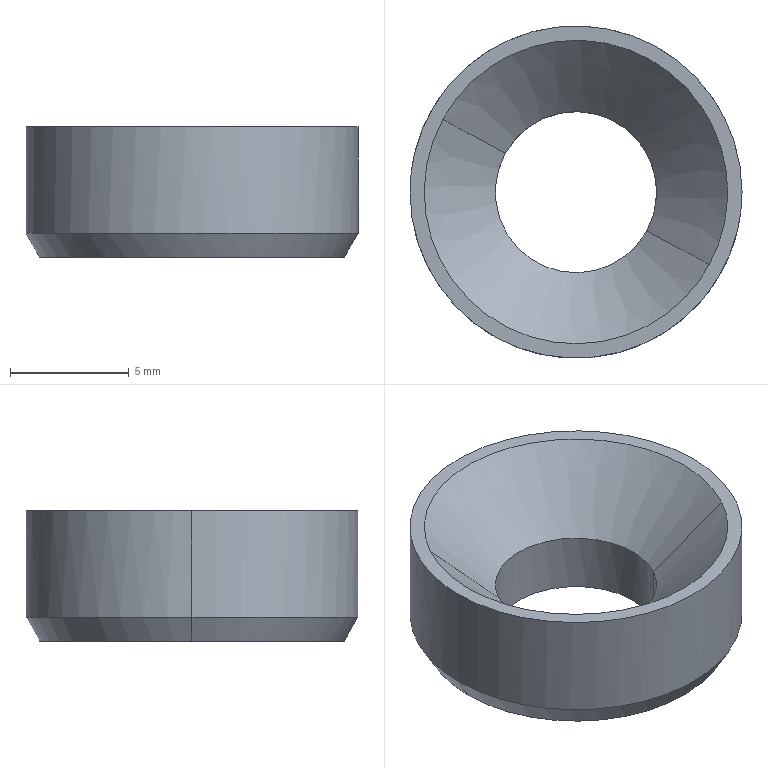Part | CATIA | 1 solid | 10 faces | box 14 x 14 x 5.5 mm | volume 510.162 mm3 | cone 4 | cylinder 4 | plane 2 | commonest cylinder face diameters 6.8 x2 14 x2
STEP:
#1=CARTESIAN_POINT('',(5.617,-3.068,5.5));
#2=VERTEX_POINT('',#1);
#3=CARTESIAN_POINT('',(-5.617,3.068,5.5));
#4=VERTEX_POINT('',#3);
#5=CARTESIAN_POINT('',(0.,0.,5.5));
#6=DIRECTION('',(0.,0.,1.));
#7=AXIS2_PLACEMENT_3D('',#5,#6,$);
#8=CIRCLE('',#7,6.4);
#9=EDGE_CURVE('',#2,#4,#8,.T.);
#10=ORIENTED_EDGE('',*,*,#9,.T.);
#11=CARTESIAN_POINT('',(-2.984,1.63,2.5));
#12=VERTEX_POINT('',#11);
#13=CARTESIAN_POINT('',(-310273.782,169503.34,353554.191));
#14=DIRECTION('',(-0.6205,0.339,0.7071));
#15=VECTOR('',#14,1.);
#16=LINE('',#13,#15);
#17=EDGE_CURVE('',#12,#4,#16,.T.);
#18=ORIENTED_EDGE('',*,*,#17,.F.);
#19=CARTESIAN_POINT('',(2.984,-1.63,2.5));
#20=VERTEX_POINT('',#19);
#21=CARTESIAN_POINT('',(0.,0.,2.5));
#22=DIRECTION('',(0.,0.,1.));
#23=AXIS2_PLACEMENT_3D('',#21,#22,$);
#24=CIRCLE('',#23,3.4);
#25=EDGE_CURVE('',#12,#20,#24,.F.);
#26=ORIENTED_EDGE('',*,*,#25,.T.);
#27=CARTESIAN_POINT('',(310273.782,-169503.34,353554.191));
#28=DIRECTION('',(0.6205,-0.339,0.7071));
#29=VECTOR('',#28,1.);
#30=LINE('',#27,#29);
#31=EDGE_CURVE('',#20,#2,#30,.T.);
#32=ORIENTED_EDGE('',*,*,#31,.T.);
#33=EDGE_LOOP('',(#10,#18,#26,#32));
#34=FACE_OUTER_BOUND('',#33,.T.);
#35=CARTESIAN_POINT('',(0.,0.,2.5));
#36=DIRECTION('',(0.,0.,1.));
#37=DIRECTION('',(0.8776,-0.4794,0.));
#38=AXIS2_PLACEMENT_3D('',#35,#36,#37);
#39=CONICAL_SURFACE('',#38,3.4,0.7854);
#40=ADVANCED_FACE('',(#34),#39,.F.);
#41=CARTESIAN_POINT('',(7.,0.,5.5));
#42=VERTEX_POINT('',#41);
#43=CARTESIAN_POINT('',(-7.,0.,5.5));
#44=VERTEX_POINT('',#43);
#45=CARTESIAN_POINT('',(7.,0.,5.5));
#46=CARTESIAN_POINT('',(7.,0.6481,5.5));
#47=CARTESIAN_POINT('',(6.925,1.296,5.5));
#48=CARTESIAN_POINT('',(6.775,1.933,5.5));
#49=CARTESIAN_POINT('',(6.33,3.159,5.5));
#50=CARTESIAN_POINT('',(5.617,4.252,5.5));
#51=CARTESIAN_POINT('',(5.199,4.755,5.5));
#52=CARTESIAN_POINT('',(4.253,5.654,5.5));
#53=CARTESIAN_POINT('',(3.127,6.313,5.5));
#54=CARTESIAN_POINT('',(2.529,6.576,5.5));
#55=CARTESIAN_POINT('',(1.281,6.958,5.5));
#56=CARTESIAN_POINT('',(-0.02086,7.045,5.5));
#57=CARTESIAN_POINT('',(-0.674,7.013,5.5));
#58=CARTESIAN_POINT('',(-1.961,6.798,5.5));
#59=CARTESIAN_POINT('',(-3.165,6.294,5.5));
#60=CARTESIAN_POINT('',(-3.735,5.974,5.5));
#61=CARTESIAN_POINT('',(-4.79,5.207,5.5));
#62=CARTESIAN_POINT('',(-5.642,4.219,5.5));
#63=CARTESIAN_POINT('',(-6.009,3.677,5.5));
#64=CARTESIAN_POINT('',(-6.547,2.643,5.5));
#65=CARTESIAN_POINT('',(-6.861,1.524,5.5));
#66=CARTESIAN_POINT('',(-6.954,1.02,5.5));
#67=CARTESIAN_POINT('',(-7.,0.5098,5.5));
#68=CARTESIAN_POINT('',(-7.,0.,5.5));
#69=B_SPLINE_CURVE_WITH_KNOTS('',5,(#45,#46,#47,#48,#49,#50,#51,#52,#53,#54,#55,#56,#57,#58,#59,#60,#61,#62,#63,#64,#65,#66,#67,#68),.UNSPECIFIED.,.F.,.U.,(6,3,3,3,3,3,3,6),(0.,4.583,9.165,13.748,18.33,22.913,27.495,31.1),.UNSPECIFIED.);
#70=EDGE_CURVE('',#42,#44,#69,.T.);
#71=ORIENTED_EDGE('',*,*,#70,.T.);
#72=CARTESIAN_POINT('',(-7.,0.,5.5));
#73=CARTESIAN_POINT('',(-7.,-0.6481,5.5));
#74=CARTESIAN_POINT('',(-6.925,-1.296,5.5));
#75=CARTESIAN_POINT('',(-6.775,-1.933,5.5));
#76=CARTESIAN_POINT('',(-6.33,-3.159,5.5));
#77=CARTESIAN_POINT('',(-5.617,-4.252,5.5));
#78=CARTESIAN_POINT('',(-5.199,-4.755,5.5));
#79=CARTESIAN_POINT('',(-4.253,-5.654,5.5));
#80=CARTESIAN_POINT('',(-3.127,-6.313,5.5));
#81=CARTESIAN_POINT('',(-2.529,-6.576,5.5));
#82=CARTESIAN_POINT('',(-1.281,-6.958,5.5));
#83=CARTESIAN_POINT('',(0.02086,-7.045,5.5));
#84=CARTESIAN_POINT('',(0.674,-7.013,5.5));
#85=CARTESIAN_POINT('',(1.961,-6.798,5.5));
#86=CARTESIAN_POINT('',(3.165,-6.294,5.5));
#87=CARTESIAN_POINT('',(3.735,-5.974,5.5));
#88=CARTESIAN_POINT('',(4.79,-5.207,5.5));
#89=CARTESIAN_POINT('',(5.642,-4.219,5.5));
#90=CARTESIAN_POINT('',(6.009,-3.677,5.5));
#91=CARTESIAN_POINT('',(6.547,-2.643,5.5));
#92=CARTESIAN_POINT('',(6.861,-1.524,5.5));
#93=CARTESIAN_POINT('',(6.954,-1.02,5.5));
#94=CARTESIAN_POINT('',(7.,-0.5098,5.5));
#95=CARTESIAN_POINT('',(7.,0.,5.5));
#96=B_SPLINE_CURVE_WITH_KNOTS('',5,(#72,#73,#74,#75,#76,#77,#78,#79,#80,#81,#82,#83,#84,#85,#86,#87,#88,#89,#90,#91,#92,#93,#94,#95),.UNSPECIFIED.,.F.,.U.,(6,3,3,3,3,3,3,6),(0.,4.583,9.165,13.748,18.33,22.913,27.495,31.1),.UNSPECIFIED.);
#97=EDGE_CURVE('',#44,#42,#96,.T.);
#98=ORIENTED_EDGE('',*,*,#97,.T.);
#99=EDGE_LOOP('',(#71,#98));
#100=FACE_OUTER_BOUND('',#99,.T.);
#101=CARTESIAN_POINT('',(-5.617,3.068,5.5));
#102=CARTESIAN_POINT('',(-5.914,2.525,5.5));
#103=CARTESIAN_POINT('',(-6.145,1.945,5.5));
#104=CARTESIAN_POINT('',(-6.305,1.34,5.5));
#105=CARTESIAN_POINT('',(-6.474,0.1028,5.5));
#106=CARTESIAN_POINT('',(-6.344,-1.139,5.5));
#107=CARTESIAN_POINT('',(-6.204,-1.749,5.5));
#108=CARTESIAN_POINT('',(-5.778,-2.922,5.5));
#109=CARTESIAN_POINT('',(-5.085,-3.961,5.5));
#110=CARTESIAN_POINT('',(-4.677,-4.435,5.5));
#111=CARTESIAN_POINT('',(-3.754,-5.276,5.5));
#112=CARTESIAN_POINT('',(-2.657,-5.872,5.5));
#113=CARTESIAN_POINT('',(-2.075,-6.102,5.5));
#114=CARTESIAN_POINT('',(-0.867,-6.417,5.5));
#115=CARTESIAN_POINT('',(0.3813,-6.434,5.5));
#116=CARTESIAN_POINT('',(1.003,-6.367,5.5));
#117=CARTESIAN_POINT('',(2.219,-6.083,5.5));
#118=CARTESIAN_POINT('',(3.332,-5.517,5.5));
#119=CARTESIAN_POINT('',(3.851,-5.168,5.5));
#120=CARTESIAN_POINT('',(4.554,-4.56,5.5));
#121=CARTESIAN_POINT('',(5.134,-3.839,5.5));
#122=CARTESIAN_POINT('',(5.31,-3.592,5.5));
#123=CARTESIAN_POINT('',(5.471,-3.334,5.5));
#124=CARTESIAN_POINT('',(5.617,-3.068,5.5));
#125=B_SPLINE_CURVE_WITH_KNOTS('',5,(#101,#102,#103,#104,#105,#106,#107,#108,#109,#110,#111,#112,#113,#114,#115,#116,#117,#118,#119,#120,#121,#122,#123,#124),.UNSPECIFIED.,.F.,.U.,(6,3,3,3,3,3,3,6),(0.,4.382,8.763,13.145,17.527,21.909,26.29,28.434),.UNSPECIFIED.);
#126=EDGE_CURVE('',#4,#2,#125,.T.);
#127=ORIENTED_EDGE('',*,*,#126,.F.);
#128=ORIENTED_EDGE('',*,*,#9,.F.);
#129=EDGE_LOOP('',(#127,#128));
#130=FACE_BOUND('',#129,.T.);
#131=CARTESIAN_POINT('',(0.,0.,5.5));
#132=DIRECTION('',(0.,0.,1.));
#133=DIRECTION('',(1.,0.,0.));
#134=AXIS2_PLACEMENT_3D('',#131,#132,#133);
#135=PLANE('',#134);
#136=ADVANCED_FACE('',(#100,#130),#135,.T.);
#137=ORIENTED_EDGE('',*,*,#126,.T.);
#138=ORIENTED_EDGE('',*,*,#31,.F.);
#139=CARTESIAN_POINT('',(0.,0.,2.5));
#140=DIRECTION('',(0.,0.,1.));
#141=AXIS2_PLACEMENT_3D('',#139,#140,$);
#142=CIRCLE('',#141,3.4);
#143=EDGE_CURVE('',#20,#12,#142,.F.);
#144=ORIENTED_EDGE('',*,*,#143,.T.);
#145=ORIENTED_EDGE('',*,*,#17,.T.);
#146=EDGE_LOOP('',(#137,#138,#144,#145));
#147=FACE_OUTER_BOUND('',#146,.T.);
#148=CARTESIAN_POINT('',(0.,0.,2.5));
#149=DIRECTION('',(0.,0.,1.));
#150=DIRECTION('',(-0.8776,0.4794,0.));
#151=AXIS2_PLACEMENT_3D('',#148,#149,#150);
#152=CONICAL_SURFACE('',#151,3.4,0.7854);
#153=ADVANCED_FACE('',(#147),#152,.F.);
#154=CARTESIAN_POINT('',(2.984,-1.63,0.));
#155=VERTEX_POINT('',#154);
#156=CARTESIAN_POINT('',(-2.984,1.63,0.));
#157=VERTEX_POINT('',#156);
#158=CARTESIAN_POINT('',(-2.984,1.63,0.));
#159=CARTESIAN_POINT('',(-2.728,2.099,0.));
#160=CARTESIAN_POINT('',(-2.38,2.517,0.));
#161=CARTESIAN_POINT('',(-1.953,2.861,0.));
#162=CARTESIAN_POINT('',(-0.9868,3.363,0.));
#163=CARTESIAN_POINT('',(0.09722,3.463,0.));
#164=CARTESIAN_POINT('',(0.6424,3.404,0.));
#165=CARTESIAN_POINT('',(1.68,3.076,0.));
#166=CARTESIAN_POINT('',(2.517,2.38,0.));
#167=CARTESIAN_POINT('',(2.861,1.953,0.));
#168=CARTESIAN_POINT('',(3.363,0.9868,0.));
#169=CARTESIAN_POINT('',(3.463,-0.09722,0.));
#170=CARTESIAN_POINT('',(3.404,-0.6424,0.));
#171=CARTESIAN_POINT('',(3.24,-1.161,0.));
#172=CARTESIAN_POINT('',(2.984,-1.63,0.));
#173=B_SPLINE_CURVE_WITH_KNOTS('',5,(#158,#159,#160,#161,#162,#163,#164,#165,#166,#167,#168,#169,#170,#171,#172),.UNSPECIFIED.,.F.,.U.,(6,3,3,3,6),(-5.341,-2.67,0.,2.67,5.341),.UNSPECIFIED.);
#174=EDGE_CURVE('',#155,#157,#173,.F.);
#175=ORIENTED_EDGE('',*,*,#174,.F.);
#176=CARTESIAN_POINT('',(2.984,-1.63,5.4));
#177=DIRECTION('',(0.,0.,-1.));
#178=VECTOR('',#177,1.);
#179=LINE('',#176,#178);
#180=EDGE_CURVE('',#155,#20,#179,.F.);
#181=ORIENTED_EDGE('',*,*,#180,.T.);
#182=ORIENTED_EDGE('',*,*,#25,.F.);
#183=CARTESIAN_POINT('',(-2.984,1.63,5.4));
#184=DIRECTION('',(0.,0.,-1.));
#185=VECTOR('',#184,1.);
#186=LINE('',#183,#185);
#187=EDGE_CURVE('',#157,#12,#186,.F.);
#188=ORIENTED_EDGE('',*,*,#187,.F.);
#189=EDGE_LOOP('',(#175,#181,#182,#188));
#190=FACE_OUTER_BOUND('',#189,.T.);
#191=CARTESIAN_POINT('',(0.,0.,5.4));
#192=DIRECTION('',(0.,0.,-1.));
#193=DIRECTION('',(-0.8776,0.4794,0.));
#194=AXIS2_PLACEMENT_3D('',#191,#192,#193);
#195=CYLINDRICAL_SURFACE('',#194,3.4);
#196=ADVANCED_FACE('',(#190),#195,.F.);
#197=CARTESIAN_POINT('',(-7.,0.,1.));
#198=VERTEX_POINT('',#197);
#199=CARTESIAN_POINT('',(-7.,0.,2.75));
#200=DIRECTION('',(0.,0.,1.));
#201=VECTOR('',#200,1.);
#202=LINE('',#199,#201);
#203=EDGE_CURVE('',#198,#44,#202,.T.);
#204=ORIENTED_EDGE('',*,*,#203,.T.);
#205=ORIENTED_EDGE('',*,*,#70,.F.);
#206=CARTESIAN_POINT('',(7.,0.,1.));
#207=VERTEX_POINT('',#206);
#208=CARTESIAN_POINT('',(7.,0.,2.75));
#209=DIRECTION('',(0.,0.,1.));
#210=VECTOR('',#209,1.);
#211=LINE('',#208,#210);
#212=EDGE_CURVE('',#207,#42,#211,.T.);
#213=ORIENTED_EDGE('',*,*,#212,.F.);
#214=CARTESIAN_POINT('',(0.,0.,1.));
#215=DIRECTION('',(0.,0.,1.));
#216=AXIS2_PLACEMENT_3D('',#214,#215,$);
#217=CIRCLE('',#216,7.);
#218=EDGE_CURVE('',#207,#198,#217,.T.);
#219=ORIENTED_EDGE('',*,*,#218,.T.);
#220=EDGE_LOOP('',(#204,#205,#213,#219));
#221=FACE_OUTER_BOUND('',#220,.T.);
#222=CARTESIAN_POINT('',(0.,0.,2.75));
#223=DIRECTION('',(0.,0.,1.));
#224=DIRECTION('',(1.,0.,0.));
#225=AXIS2_PLACEMENT_3D('',#222,#223,#224);
#226=CYLINDRICAL_SURFACE('',#225,7.);
#227=ADVANCED_FACE('',(#221),#226,.T.);
#228=ORIENTED_EDGE('',*,*,#212,.T.);
#229=ORIENTED_EDGE('',*,*,#97,.F.);
#230=ORIENTED_EDGE('',*,*,#203,.F.);
#231=CARTESIAN_POINT('',(0.,0.,1.));
#232=DIRECTION('',(0.,0.,1.));
#233=AXIS2_PLACEMENT_3D('',#231,#232,$);
#234=CIRCLE('',#233,7.);
#235=EDGE_CURVE('',#198,#207,#234,.T.);
#236=ORIENTED_EDGE('',*,*,#235,.T.);
#237=EDGE_LOOP('',(#228,#229,#230,#236));
#238=FACE_OUTER_BOUND('',#237,.T.);
#239=CARTESIAN_POINT('',(0.,0.,2.75));
#240=DIRECTION('',(0.,0.,1.));
#241=DIRECTION('',(-1.,0.,0.));
#242=AXIS2_PLACEMENT_3D('',#239,#240,#241);
#243=CYLINDRICAL_SURFACE('',#242,7.);
#244=ADVANCED_FACE('',(#238),#243,.T.);
#245=CARTESIAN_POINT('',(0.,0.,0.));
#246=DIRECTION('',(0.,0.,-1.));
#247=AXIS2_PLACEMENT_3D('',#245,#246,$);
#248=CIRCLE('',#247,3.4);
#249=EDGE_CURVE('',#157,#155,#248,.F.);
#250=ORIENTED_EDGE('',*,*,#249,.F.);
#251=ORIENTED_EDGE('',*,*,#187,.T.);
#252=ORIENTED_EDGE('',*,*,#143,.F.);
#253=ORIENTED_EDGE('',*,*,#180,.F.);
#254=EDGE_LOOP('',(#250,#251,#252,#253));
#255=FACE_OUTER_BOUND('',#254,.T.);
#256=CARTESIAN_POINT('',(0.,0.,5.4));
#257=DIRECTION('',(0.,0.,-1.));
#258=DIRECTION('',(0.8776,-0.4794,0.));
#259=AXIS2_PLACEMENT_3D('',#256,#257,#258);
#260=CYLINDRICAL_SURFACE('',#259,3.4);
#261=ADVANCED_FACE('',(#255),#260,.F.);
#262=CARTESIAN_POINT('',(-6.423,0.000000049,0.));
#263=VERTEX_POINT('',#262);
#264=CARTESIAN_POINT('',(6.423,0.,0.));
#265=VERTEX_POINT('',#264);
#266=CARTESIAN_POINT('',(-6.423,0.000000048,0.));
#267=CARTESIAN_POINT('',(-6.423,-0.6208,0.));
#268=CARTESIAN_POINT('',(-6.348,-1.242,0.));
#269=CARTESIAN_POINT('',(-6.198,-1.85,0.));
#270=CARTESIAN_POINT('',(-5.754,-3.019,0.));
#271=CARTESIAN_POINT('',(-5.044,-4.049,0.));
#272=CARTESIAN_POINT('',(-4.628,-4.518,0.));
#273=CARTESIAN_POINT('',(-3.692,-5.347,0.));
#274=CARTESIAN_POINT('',(-2.585,-5.929,0.));
#275=CARTESIAN_POINT('',(-1.999,-6.151,0.));
#276=CARTESIAN_POINT('',(-0.7842,-6.45,0.));
#277=CARTESIAN_POINT('',(0.4663,-6.451,0.));
#278=CARTESIAN_POINT('',(1.089,-6.376,0.));
#279=CARTESIAN_POINT('',(2.303,-6.076,0.));
#280=CARTESIAN_POINT('',(3.411,-5.496,0.));
#281=CARTESIAN_POINT('',(3.927,-5.14,0.));
#282=CARTESIAN_POINT('',(4.862,-4.31,0.));
#283=CARTESIAN_POINT('',(5.574,-3.281,0.));
#284=CARTESIAN_POINT('',(5.865,-2.726,0.));
#285=CARTESIAN_POINT('',(6.198,-1.849,0.));
#286=CARTESIAN_POINT('',(6.366,-0.931,0.));
#287=CARTESIAN_POINT('',(6.404,-0.6217,0.));
#288=CARTESIAN_POINT('',(6.423,-0.3108,0.));
#289=CARTESIAN_POINT('',(6.423,0.,0.));
#290=B_SPLINE_CURVE_WITH_KNOTS('',5,(#266,#267,#268,#269,#270,#271,#272,#273,#274,#275,#276,#277,#278,#279,#280,#281,#282,#283,#284,#285,#286,#287,#288,#289),.UNSPECIFIED.,.F.,.U.,(6,3,3,3,3,3,3,6),(0.,4.389,8.779,13.168,17.558,21.947,26.337,28.535),.UNSPECIFIED.);
#291=EDGE_CURVE('',#263,#265,#290,.T.);
#292=ORIENTED_EDGE('',*,*,#291,.F.);
#293=CARTESIAN_POINT('',(6.423,0.,0.));
#294=CARTESIAN_POINT('',(6.423,0.6208,0.));
#295=CARTESIAN_POINT('',(6.348,1.242,0.));
#296=CARTESIAN_POINT('',(6.198,1.85,0.));
#297=CARTESIAN_POINT('',(5.754,3.019,0.));
#298=CARTESIAN_POINT('',(5.044,4.049,0.));
#299=CARTESIAN_POINT('',(4.628,4.518,0.));
#300=CARTESIAN_POINT('',(3.692,5.347,0.));
#301=CARTESIAN_POINT('',(2.585,5.929,0.));
#302=CARTESIAN_POINT('',(1.999,6.151,0.));
#303=CARTESIAN_POINT('',(0.7842,6.45,0.));
#304=CARTESIAN_POINT('',(-0.4663,6.451,0.));
#305=CARTESIAN_POINT('',(-1.089,6.376,0.));
#306=CARTESIAN_POINT('',(-2.303,6.076,0.));
#307=CARTESIAN_POINT('',(-3.411,5.496,0.));
#308=CARTESIAN_POINT('',(-3.927,5.14,0.));
#309=CARTESIAN_POINT('',(-4.862,4.31,0.));
#310=CARTESIAN_POINT('',(-5.574,3.281,0.));
#311=CARTESIAN_POINT('',(-5.865,2.726,0.));
#312=CARTESIAN_POINT('',(-6.198,1.849,0.));
#313=CARTESIAN_POINT('',(-6.366,0.931,0.));
#314=CARTESIAN_POINT('',(-6.404,0.6217,0.));
#315=CARTESIAN_POINT('',(-6.423,0.3108,0.));
#316=CARTESIAN_POINT('',(-6.423,0.000000048,0.));
#317=B_SPLINE_CURVE_WITH_KNOTS('',5,(#293,#294,#295,#296,#297,#298,#299,#300,#301,#302,#303,#304,#305,#306,#307,#308,#309,#310,#311,#312,#313,#314,#315,#316),.UNSPECIFIED.,.F.,.U.,(6,3,3,3,3,3,3,6),(0.,4.389,8.779,13.168,17.558,21.947,26.337,28.535),.UNSPECIFIED.);
#318=EDGE_CURVE('',#265,#263,#317,.T.);
#319=ORIENTED_EDGE('',*,*,#318,.F.);
#320=EDGE_LOOP('',(#292,#319));
#321=FACE_OUTER_BOUND('',#320,.T.);
#322=ORIENTED_EDGE('',*,*,#174,.T.);
#323=ORIENTED_EDGE('',*,*,#249,.T.);
#324=EDGE_LOOP('',(#322,#323));
#325=FACE_BOUND('',#324,.T.);
#326=CARTESIAN_POINT('',(0.,0.,0.));
#327=DIRECTION('',(0.,0.,1.));
#328=DIRECTION('',(1.,0.,0.));
#329=AXIS2_PLACEMENT_3D('',#326,#327,#328);
#330=PLANE('',#329);
#331=ADVANCED_FACE('',(#321,#325),#330,.F.);
#332=CARTESIAN_POINT('',(250000.,0.000000001,433001.578));
#333=DIRECTION('',(0.5,0.,0.866));
#334=VECTOR('',#333,1.);
#335=LINE('',#332,#334);
#336=EDGE_CURVE('',#207,#265,#335,.F.);
#337=ORIENTED_EDGE('',*,*,#336,.T.);
#338=ORIENTED_EDGE('',*,*,#318,.T.);
#339=CARTESIAN_POINT('',(-250000.,0.000000001,433001.578));
#340=DIRECTION('',(-0.5,0.,0.866));
#341=VECTOR('',#340,1.);
#342=LINE('',#339,#341);
#343=EDGE_CURVE('',#198,#263,#342,.F.);
#344=ORIENTED_EDGE('',*,*,#343,.F.);
#345=ORIENTED_EDGE('',*,*,#218,.F.);
#346=EDGE_LOOP('',(#337,#338,#344,#345));
#347=FACE_OUTER_BOUND('',#346,.T.);
#348=CARTESIAN_POINT('',(0.,0.,-11.124));
#349=DIRECTION('',(0.,0.,1.));
#350=DIRECTION('',(1.,0.,0.));
#351=AXIS2_PLACEMENT_3D('',#348,#349,#350);
#352=CONICAL_SURFACE('',#351,0.,0.5236);
#353=ADVANCED_FACE('',(#347),#352,.T.);
#354=ORIENTED_EDGE('',*,*,#343,.T.);
#355=ORIENTED_EDGE('',*,*,#291,.T.);
#356=ORIENTED_EDGE('',*,*,#336,.F.);
#357=ORIENTED_EDGE('',*,*,#235,.F.);
#358=EDGE_LOOP('',(#354,#355,#356,#357));
#359=FACE_OUTER_BOUND('',#358,.T.);
#360=CARTESIAN_POINT('',(0.,0.,-11.124));
#361=DIRECTION('',(0.,0.,1.));
#362=DIRECTION('',(-1.,0.,0.));
#363=AXIS2_PLACEMENT_3D('',#360,#361,#362);
#364=CONICAL_SURFACE('',#363,0.,0.5236);
#365=ADVANCED_FACE('',(#359),#364,.T.);
#366=CLOSED_SHELL('',(#40,#136,#153,#196,#227,#244,#261,#331,#353,#365));
#367=MANIFOLD_SOLID_BREP('',#366);
#368=(LENGTH_UNIT()NAMED_UNIT(*)SI_UNIT(.MILLI.,.METRE.));
#369=UNCERTAINTY_MEASURE_WITH_UNIT(LENGTH_MEASURE(0.005),#368,'','');
#370=(NAMED_UNIT(*)PLANE_ANGLE_UNIT()SI_UNIT($,.RADIAN.));
#371=(NAMED_UNIT(*)SI_UNIT($,.STERADIAN.)SOLID_ANGLE_UNIT());
#372=(GEOMETRIC_REPRESENTATION_CONTEXT(3)GLOBAL_UNCERTAINTY_ASSIGNED_CONTEXT((#369))GLOBAL_UNIT_ASSIGNED_CONTEXT((#368,#370,#371))REPRESENTATION_CONTEXT('',''));
#373=ADVANCED_BREP_SHAPE_REPRESENTATION('',(#367),#372);